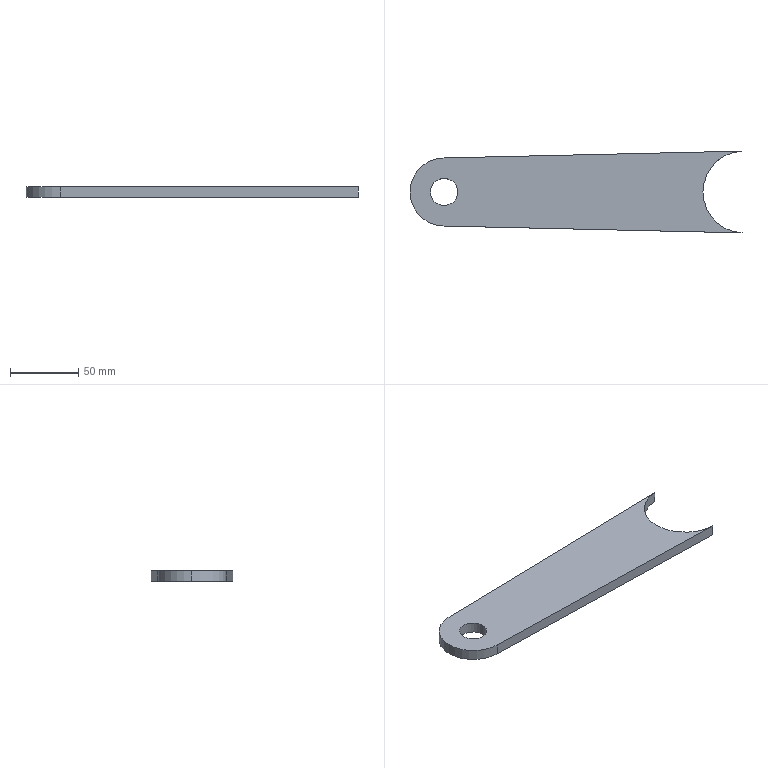Part | SolidWorks | features Extrusion 1, ICE 1 | 1 solid | 10 faces | box 243.637 x 59.938 x 8 mm | volume 90831 mm3 | cylinder 6 | plane 4 | commonest cylinder face diameters 20 x2 50 x2 60 x2
STEP:
#1=CARTESIAN_POINT('',(-10.,0.,0.));
#2=VERTEX_POINT('',#1);
#3=CARTESIAN_POINT('',(10.,0.,0.));
#4=VERTEX_POINT('',#3);
#5=CARTESIAN_POINT('',(0.,0.,0.));
#6=DIRECTION('',(0.,0.,1.));
#7=DIRECTION('',(1.,0.,0.));
#8=AXIS2_PLACEMENT_3D('',#5,#6,#7);
#9=CIRCLE('',#8,10.);
#10=EDGE_CURVE('',#2,#4,#9,.T.);
#11=ORIENTED_EDGE('',*,*,#10,.F.);
#12=CARTESIAN_POINT('',(-10.,0.,8.));
#13=VERTEX_POINT('',#12);
#14=CARTESIAN_POINT('',(-10.,0.,0.));
#15=DIRECTION('',(0.,0.,1.));
#16=VECTOR('',#15,1000.);
#17=LINE('',#14,#16);
#18=EDGE_CURVE('',#2,#13,#17,.T.);
#19=ORIENTED_EDGE('',*,*,#18,.T.);
#20=CARTESIAN_POINT('',(10.,0.,8.));
#21=VERTEX_POINT('',#20);
#22=CARTESIAN_POINT('',(0.,0.,8.));
#23=DIRECTION('',(0.,0.,1.));
#24=DIRECTION('',(1.,0.,0.));
#25=AXIS2_PLACEMENT_3D('',#22,#23,#24);
#26=CIRCLE('',#25,10.);
#27=EDGE_CURVE('',#13,#21,#26,.T.);
#28=ORIENTED_EDGE('',*,*,#27,.T.);
#29=CARTESIAN_POINT('',(10.,0.,0.));
#30=DIRECTION('',(0.,0.,1.));
#31=VECTOR('',#30,1000.);
#32=LINE('',#29,#31);
#33=EDGE_CURVE('',#4,#21,#32,.T.);
#34=ORIENTED_EDGE('',*,*,#33,.F.);
#35=EDGE_LOOP('',(#11,#19,#28,#34));
#36=FACE_OUTER_BOUND('',#35,.T.);
#37=CARTESIAN_POINT('',(0.,0.,0.));
#38=DIRECTION('',(0.,0.,1.));
#39=DIRECTION('',(1.,0.,0.));
#40=AXIS2_PLACEMENT_3D('',#37,#38,#39);
#41=CYLINDRICAL_SURFACE('',#40,10.);
#42=ADVANCED_FACE('',(#36),#41,.F.);
#43=CARTESIAN_POINT('',(-25.,0.,8.));
#44=VERTEX_POINT('',#43);
#45=CARTESIAN_POINT('',(0.,-25.,8.));
#46=VERTEX_POINT('',#45);
#47=CARTESIAN_POINT('',(0.,0.,8.));
#48=DIRECTION('',(0.,0.,1.));
#49=DIRECTION('',(1.,0.,0.));
#50=AXIS2_PLACEMENT_3D('',#47,#48,#49);
#51=CIRCLE('',#50,25.);
#52=EDGE_CURVE('',#44,#46,#51,.T.);
#53=ORIENTED_EDGE('',*,*,#52,.F.);
#54=CARTESIAN_POINT('',(-25.,0.,0.));
#55=VERTEX_POINT('',#54);
#56=CARTESIAN_POINT('',(-25.,0.,8.));
#57=DIRECTION('',(0.,0.,-1.));
#58=VECTOR('',#57,1000.);
#59=LINE('',#56,#58);
#60=EDGE_CURVE('',#44,#55,#59,.T.);
#61=ORIENTED_EDGE('',*,*,#60,.T.);
#62=CARTESIAN_POINT('',(0.,-25.,0.));
#63=VERTEX_POINT('',#62);
#64=CARTESIAN_POINT('',(0.,0.,0.));
#65=DIRECTION('',(0.,0.,1.));
#66=DIRECTION('',(1.,0.,0.));
#67=AXIS2_PLACEMENT_3D('',#64,#65,#66);
#68=CIRCLE('',#67,25.);
#69=EDGE_CURVE('',#55,#63,#68,.T.);
#70=ORIENTED_EDGE('',*,*,#69,.T.);
#71=CARTESIAN_POINT('',(0.,-25.,8.));
#72=DIRECTION('',(0.,0.,-1.));
#73=VECTOR('',#72,1000.);
#74=LINE('',#71,#73);
#75=EDGE_CURVE('',#46,#63,#74,.T.);
#76=ORIENTED_EDGE('',*,*,#75,.F.);
#77=EDGE_LOOP('',(#53,#61,#70,#76));
#78=FACE_OUTER_BOUND('',#77,.T.);
#79=CARTESIAN_POINT('',(0.,0.,8.));
#80=DIRECTION('',(0.,0.,-1.));
#81=DIRECTION('',(-1.,0.,0.));
#82=AXIS2_PLACEMENT_3D('',#79,#80,#81);
#83=CYLINDRICAL_SURFACE('',#82,25.);
#84=ADVANCED_FACE('',(#78),#83,.T.);
#85=CARTESIAN_POINT('',(218.637,29.969,8.));
#86=VERTEX_POINT('',#85);
#87=CARTESIAN_POINT('',(190.,0.,8.));
#88=VERTEX_POINT('',#87);
#89=CARTESIAN_POINT('',(220.,0.,8.));
#90=DIRECTION('',(0.,0.,1.));
#91=DIRECTION('',(1.,0.,0.));
#92=AXIS2_PLACEMENT_3D('',#89,#90,#91);
#93=CIRCLE('',#92,30.);
#94=EDGE_CURVE('',#86,#88,#93,.T.);
#95=ORIENTED_EDGE('',*,*,#94,.T.);
#96=CARTESIAN_POINT('',(190.,0.,0.));
#97=VERTEX_POINT('',#96);
#98=CARTESIAN_POINT('',(190.,0.,8.));
#99=DIRECTION('',(0.,0.,-1.));
#100=VECTOR('',#99,1000.);
#101=LINE('',#98,#100);
#102=EDGE_CURVE('',#88,#97,#101,.T.);
#103=ORIENTED_EDGE('',*,*,#102,.T.);
#104=CARTESIAN_POINT('',(218.637,29.969,0.));
#105=VERTEX_POINT('',#104);
#106=CARTESIAN_POINT('',(220.,0.,0.));
#107=DIRECTION('',(0.,0.,1.));
#108=DIRECTION('',(1.,0.,0.));
#109=AXIS2_PLACEMENT_3D('',#106,#107,#108);
#110=CIRCLE('',#109,30.);
#111=EDGE_CURVE('',#105,#97,#110,.T.);
#112=ORIENTED_EDGE('',*,*,#111,.F.);
#113=CARTESIAN_POINT('',(218.637,29.969,8.));
#114=DIRECTION('',(0.,0.,-1.));
#115=VECTOR('',#114,1000.);
#116=LINE('',#113,#115);
#117=EDGE_CURVE('',#86,#105,#116,.T.);
#118=ORIENTED_EDGE('',*,*,#117,.F.);
#119=EDGE_LOOP('',(#95,#103,#112,#118));
#120=FACE_OUTER_BOUND('',#119,.T.);
#121=CARTESIAN_POINT('',(220.,0.,8.));
#122=DIRECTION('',(0.,0.,-1.));
#123=DIRECTION('',(-1.,0.,0.));
#124=AXIS2_PLACEMENT_3D('',#121,#122,#123);
#125=CYLINDRICAL_SURFACE('',#124,30.);
#126=ADVANCED_FACE('',(#120),#125,.F.);
#127=ORIENTED_EDGE('',*,*,#102,.F.);
#128=CARTESIAN_POINT('',(218.637,-29.969,8.));
#129=VERTEX_POINT('',#128);
#130=CARTESIAN_POINT('',(220.,0.,8.));
#131=DIRECTION('',(0.,0.,1.));
#132=DIRECTION('',(1.,0.,0.));
#133=AXIS2_PLACEMENT_3D('',#130,#131,#132);
#134=CIRCLE('',#133,30.);
#135=EDGE_CURVE('',#88,#129,#134,.T.);
#136=ORIENTED_EDGE('',*,*,#135,.T.);
#137=CARTESIAN_POINT('',(218.637,-29.969,0.));
#138=VERTEX_POINT('',#137);
#139=CARTESIAN_POINT('',(218.637,-29.969,8.));
#140=DIRECTION('',(0.,0.,-1.));
#141=VECTOR('',#140,1000.);
#142=LINE('',#139,#141);
#143=EDGE_CURVE('',#129,#138,#142,.T.);
#144=ORIENTED_EDGE('',*,*,#143,.T.);
#145=CARTESIAN_POINT('',(220.,0.,0.));
#146=DIRECTION('',(0.,0.,1.));
#147=DIRECTION('',(1.,0.,0.));
#148=AXIS2_PLACEMENT_3D('',#145,#146,#147);
#149=CIRCLE('',#148,30.);
#150=EDGE_CURVE('',#97,#138,#149,.T.);
#151=ORIENTED_EDGE('',*,*,#150,.F.);
#152=EDGE_LOOP('',(#127,#136,#144,#151));
#153=FACE_OUTER_BOUND('',#152,.T.);
#154=CARTESIAN_POINT('',(220.,0.,8.));
#155=DIRECTION('',(0.,0.,-1.));
#156=DIRECTION('',(-1.,0.,0.));
#157=AXIS2_PLACEMENT_3D('',#154,#155,#156);
#158=CYLINDRICAL_SURFACE('',#157,30.);
#159=ADVANCED_FACE('',(#153),#158,.F.);
#160=CARTESIAN_POINT('',(0.,25.,0.));
#161=VERTEX_POINT('',#160);
#162=CARTESIAN_POINT('',(-0.5679,24.987,0.));
#163=DIRECTION('',(0.9997,0.02272,0.));
#164=VECTOR('',#163,1000.);
#165=LINE('',#162,#164);
#166=EDGE_CURVE('',#161,#105,#165,.T.);
#167=ORIENTED_EDGE('',*,*,#166,.F.);
#168=CARTESIAN_POINT('',(0.,25.,8.));
#169=VERTEX_POINT('',#168);
#170=CARTESIAN_POINT('',(0.,25.,8.));
#171=DIRECTION('',(0.,0.,-1.));
#172=VECTOR('',#171,1000.);
#173=LINE('',#170,#172);
#174=EDGE_CURVE('',#169,#161,#173,.T.);
#175=ORIENTED_EDGE('',*,*,#174,.F.);
#176=CARTESIAN_POINT('',(-0.5679,24.987,8.));
#177=DIRECTION('',(0.9997,0.02272,0.));
#178=VECTOR('',#177,1000.);
#179=LINE('',#176,#178);
#180=EDGE_CURVE('',#169,#86,#179,.T.);
#181=ORIENTED_EDGE('',*,*,#180,.T.);
#182=ORIENTED_EDGE('',*,*,#117,.T.);
#183=EDGE_LOOP('',(#167,#175,#181,#182));
#184=FACE_OUTER_BOUND('',#183,.T.);
#185=CARTESIAN_POINT('',(-0.5679,24.987,8.));
#186=DIRECTION('',(-0.02272,0.9997,0.));
#187=DIRECTION('',(-0.9997,-0.02272,0.));
#188=AXIS2_PLACEMENT_3D('',#185,#186,#187);
#189=PLANE('',#188);
#190=ADVANCED_FACE('',(#184),#189,.T.);
#191=ORIENTED_EDGE('',*,*,#60,.F.);
#192=CARTESIAN_POINT('',(0.,0.,8.));
#193=DIRECTION('',(0.,0.,1.));
#194=DIRECTION('',(1.,0.,0.));
#195=AXIS2_PLACEMENT_3D('',#192,#193,#194);
#196=CIRCLE('',#195,25.);
#197=EDGE_CURVE('',#169,#44,#196,.T.);
#198=ORIENTED_EDGE('',*,*,#197,.F.);
#199=ORIENTED_EDGE('',*,*,#174,.T.);
#200=CARTESIAN_POINT('',(0.,0.,0.));
#201=DIRECTION('',(0.,0.,1.));
#202=DIRECTION('',(1.,0.,0.));
#203=AXIS2_PLACEMENT_3D('',#200,#201,#202);
#204=CIRCLE('',#203,25.);
#205=EDGE_CURVE('',#161,#55,#204,.T.);
#206=ORIENTED_EDGE('',*,*,#205,.T.);
#207=EDGE_LOOP('',(#191,#198,#199,#206));
#208=FACE_OUTER_BOUND('',#207,.T.);
#209=CARTESIAN_POINT('',(0.,0.,8.));
#210=DIRECTION('',(0.,0.,-1.));
#211=DIRECTION('',(-1.,0.,0.));
#212=AXIS2_PLACEMENT_3D('',#209,#210,#211);
#213=CYLINDRICAL_SURFACE('',#212,25.);
#214=ADVANCED_FACE('',(#208),#213,.T.);
#215=CARTESIAN_POINT('',(-0.5679,-24.987,0.));
#216=DIRECTION('',(-0.9997,0.02272,0.));
#217=VECTOR('',#216,1000.);
#218=LINE('',#215,#217);
#219=EDGE_CURVE('',#138,#63,#218,.T.);
#220=ORIENTED_EDGE('',*,*,#219,.F.);
#221=ORIENTED_EDGE('',*,*,#143,.F.);
#222=CARTESIAN_POINT('',(-0.5679,-24.987,8.));
#223=DIRECTION('',(-0.9997,0.02272,0.));
#224=VECTOR('',#223,1000.);
#225=LINE('',#222,#224);
#226=EDGE_CURVE('',#129,#46,#225,.T.);
#227=ORIENTED_EDGE('',*,*,#226,.T.);
#228=ORIENTED_EDGE('',*,*,#75,.T.);
#229=EDGE_LOOP('',(#220,#221,#227,#228));
#230=FACE_OUTER_BOUND('',#229,.T.);
#231=CARTESIAN_POINT('',(-0.5679,-24.987,8.));
#232=DIRECTION('',(-0.02272,-0.9997,0.));
#233=DIRECTION('',(0.9997,-0.02272,0.));
#234=AXIS2_PLACEMENT_3D('',#231,#232,#233);
#235=PLANE('',#234);
#236=ADVANCED_FACE('',(#230),#235,.T.);
#237=CARTESIAN_POINT('',(0.,0.,8.));
#238=DIRECTION('',(0.,0.,1.));
#239=DIRECTION('',(1.,0.,0.));
#240=AXIS2_PLACEMENT_3D('',#237,#238,#239);
#241=CIRCLE('',#240,10.);
#242=EDGE_CURVE('',#21,#13,#241,.T.);
#243=ORIENTED_EDGE('',*,*,#242,.F.);
#244=ORIENTED_EDGE('',*,*,#27,.F.);
#245=EDGE_LOOP('',(#243,#244));
#246=FACE_BOUND('',#245,.T.);
#247=ORIENTED_EDGE('',*,*,#94,.F.);
#248=ORIENTED_EDGE('',*,*,#180,.F.);
#249=ORIENTED_EDGE('',*,*,#197,.T.);
#250=ORIENTED_EDGE('',*,*,#52,.T.);
#251=ORIENTED_EDGE('',*,*,#226,.F.);
#252=ORIENTED_EDGE('',*,*,#135,.F.);
#253=EDGE_LOOP('',(#247,#248,#249,#250,#251,#252));
#254=FACE_OUTER_BOUND('',#253,.T.);
#255=CARTESIAN_POINT('',(0.,0.,8.));
#256=DIRECTION('',(0.,0.,1.));
#257=DIRECTION('',(1.,0.,0.));
#258=AXIS2_PLACEMENT_3D('',#255,#256,#257);
#259=PLANE('',#258);
#260=ADVANCED_FACE('',(#246,#254),#259,.T.);
#261=CARTESIAN_POINT('',(0.,0.,0.));
#262=DIRECTION('',(0.,0.,1.));
#263=DIRECTION('',(1.,0.,0.));
#264=AXIS2_PLACEMENT_3D('',#261,#262,#263);
#265=CIRCLE('',#264,10.);
#266=EDGE_CURVE('',#4,#2,#265,.T.);
#267=ORIENTED_EDGE('',*,*,#266,.T.);
#268=ORIENTED_EDGE('',*,*,#10,.T.);
#269=EDGE_LOOP('',(#267,#268));
#270=FACE_BOUND('',#269,.T.);
#271=ORIENTED_EDGE('',*,*,#111,.T.);
#272=ORIENTED_EDGE('',*,*,#150,.T.);
#273=ORIENTED_EDGE('',*,*,#219,.T.);
#274=ORIENTED_EDGE('',*,*,#69,.F.);
#275=ORIENTED_EDGE('',*,*,#205,.F.);
#276=ORIENTED_EDGE('',*,*,#166,.T.);
#277=EDGE_LOOP('',(#271,#272,#273,#274,#275,#276));
#278=FACE_OUTER_BOUND('',#277,.T.);
#279=CARTESIAN_POINT('',(0.,0.,0.));
#280=DIRECTION('',(0.,0.,1.));
#281=DIRECTION('',(1.,0.,0.));
#282=AXIS2_PLACEMENT_3D('',#279,#280,#281);
#283=PLANE('',#282);
#284=ADVANCED_FACE('',(#270,#278),#283,.F.);
#285=ORIENTED_EDGE('',*,*,#18,.F.);
#286=ORIENTED_EDGE('',*,*,#266,.F.);
#287=ORIENTED_EDGE('',*,*,#33,.T.);
#288=ORIENTED_EDGE('',*,*,#242,.T.);
#289=EDGE_LOOP('',(#285,#286,#287,#288));
#290=FACE_OUTER_BOUND('',#289,.T.);
#291=CARTESIAN_POINT('',(0.,0.,0.));
#292=DIRECTION('',(0.,0.,1.));
#293=DIRECTION('',(1.,0.,0.));
#294=AXIS2_PLACEMENT_3D('',#291,#292,#293);
#295=CYLINDRICAL_SURFACE('',#294,10.);
#296=ADVANCED_FACE('',(#290),#295,.F.);
#297=CLOSED_SHELL('',(#42,#84,#126,#159,#190,#214,#236,#260,#284,#296));
#298=MANIFOLD_SOLID_BREP('',#297);
#299=CARTESIAN_POINT('',(0.,0.,0.));
#300=DIRECTION('',(0.,0.,1.));
#301=DIRECTION('',(1.,0.,0.));
#302=AXIS2_PLACEMENT_3D('',#299,#300,#301);
#303=(LENGTH_UNIT()NAMED_UNIT(*)SI_UNIT(.MILLI.,.METRE.));
#304=UNCERTAINTY_MEASURE_WITH_UNIT(LENGTH_MEASURE(0.00001),#303,'','');
#305=(NAMED_UNIT(*)PLANE_ANGLE_UNIT()SI_UNIT($,.RADIAN.));
#306=(NAMED_UNIT(*)SI_UNIT($,.STERADIAN.)SOLID_ANGLE_UNIT());
#307=(GEOMETRIC_REPRESENTATION_CONTEXT(3)GLOBAL_UNCERTAINTY_ASSIGNED_CONTEXT((#304))GLOBAL_UNIT_ASSIGNED_CONTEXT((#303,#305,#306))REPRESENTATION_CONTEXT('',''));
#308=ADVANCED_BREP_SHAPE_REPRESENTATION('',(#298,#302),#307);